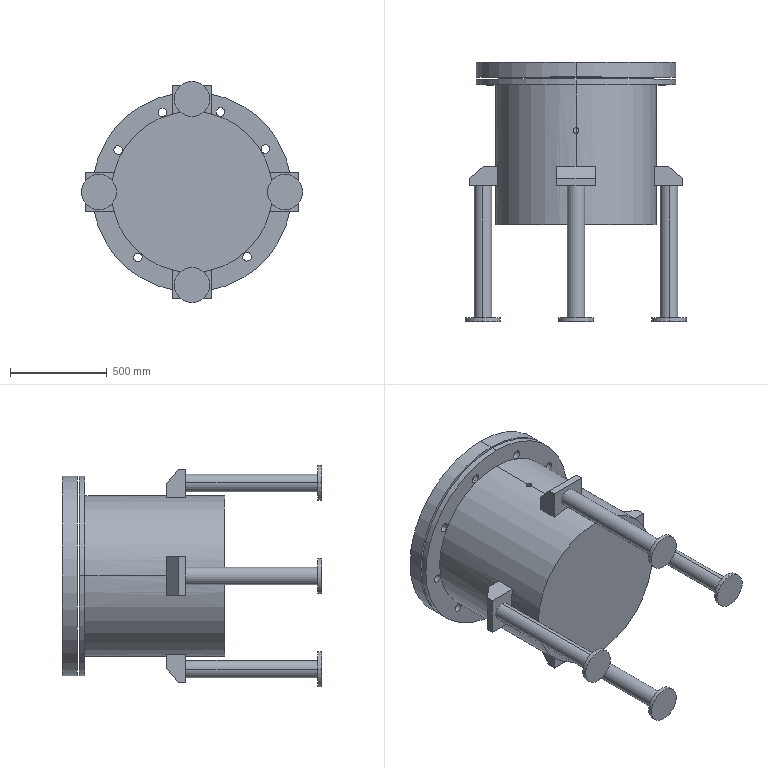Part | SolidWorks | features ICE 10, CirPattern 2, 3DProfileFeature 1, Extrusion 1, Shell 1 | 5 solids | 238 faces | box 1141 x 1336 x 1141 mm | volume 298249158 mm3 | cylinder 156 | plane 82 | commonest cylinder face diameters 44.371 x90 90 x16 180.752 x16 1030 x10 30 x8 800 x8